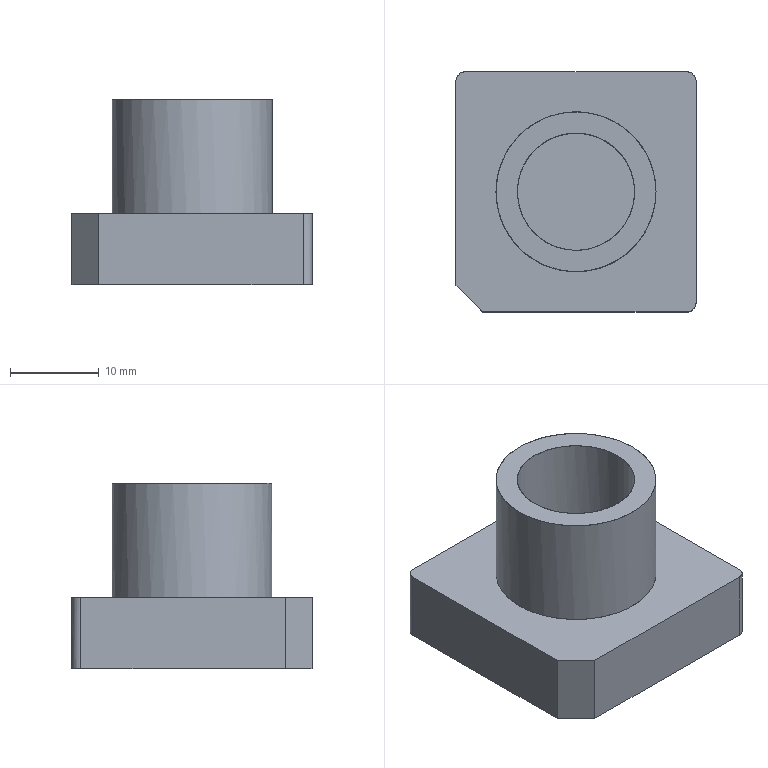NC program | PowerMill | posted with a generic post | part box 27 x 27 x 20.913 mm
Lines 15961 to 16766 of 92133:
N16058 M6
N16059 S8500 M03
N16060 G00 G90 X0.0 Y0.0
N16061 G43 Z11.803 H3
N16062
N16063 G05 P10000 R8
N16064 X19.2087 Y-4.6129
N16065 Z0.9326
N16066 G01 Z-0.2674 F360.0
N16067 X14.0835 Y-3.3645 F600.0
N16068 X1.7775 Y14.3702
N16069 X1.7498 Y14.3737
N16070 G03 X0.8293 Y14.4547 I-1.6397 J-13.3537
N16071 G01 X0.4792 Y14.472
N16072 G03 X-0.4792 I-0.4792 J-16.9289
N16073 G01 X-1.1152 Y14.4364
N16074 G03 X-2.0169 Y14.338 I1.0076 J-13.414
N16075 G01 X-2.3861 Y14.282
N16076 X-3.0221 Y14.1611
N16077 X-3.7382 Y13.9889
N16078 X-3.8175 Y13.9674
N16079 X11.7477 Y-8.4641
N16080 X11.5276 Y-8.7591
N16081 X11.3004 Y-9.0526
N16082 X11.0316 Y-9.379
N16083 X10.6658 Y-9.7933
N16084 X10.4003 Y-10.073
N16085 X10.1293 Y-10.3473
N16086 X9.7958 Y-10.6635
N16087 X9.4375 Y-10.9818
N16088 X9.0741 Y-11.284
N16089 X8.7582 Y-11.5288
N16090 X8.4375 Y-11.7672
N16091 X8.2539 Y-11.8951
N16092 X-8.2539 Y11.8951
N16093 X-8.4375 Y11.7672
N16094 X-8.7582 Y11.5288
N16095 X-9.0741 Y11.284
N16096 X-9.4375 Y10.9818
N16097 X-9.7958 Y10.6635
N16098 X-10.1293 Y10.3473
N16099 X-10.4003 Y10.073
N16100 X-10.6658 Y9.7933
N16101 X-11.0337 Y9.3766
N16102 X-11.2701 Y9.0893
N16103 X-11.6227 Y8.634
N16104 X-11.7476 Y8.464
N16105 X3.8175 Y-13.9674
N16106 X3.3294 Y-14.0906
N16107 X2.9954 Y-14.1667
N16108 X2.3861 Y-14.282
N16109 X2.0169 Y-14.338
N16110 G02 X1.1152 Y-14.4364 I-1.9093 J13.3156
N16111 G01 X0.4792 Y-14.472
N16112 G02 X-0.4792 I-0.4792 J16.9289
N16113 G01 X-0.8293 Y-14.4547
N16114 G02 X-1.7498 Y-14.3737 I0.7192 J13.4347
N16115 G01 X-1.7775 Y-14.3702
N16116 X-14.0835 Y3.3645
N16117 G00 Z11.803
N16118 G05 P0
N16119 (---------------)
N16120 ( END TOOLPATH : 精公基准台01-平坦面平行-D10 )
N16121 (---------------)
N16122 ( START TOOLPATH : 精公基准台01-基准面偏置-D10 )
N16123 (---------------)
N16124 G00 X0.0 Y0.0 Z9.8026
N16125 G05 P10000 R8
N16126 X8.5669 Y-24.255
N16127 Z-11.91
N16128 G01 Z-13.11 F360.0
N16129 Y-18.98 F600.0
N16130 X10.992 Y-9.2715
N16131 X10.7303 Y-9.5708
N16132 X10.4625 Y-9.8647
N16133 X10.1631 Y-10.1736
N16134 X9.8647 Y-10.4616
N16135 X9.5828 Y-10.7217
N16136 X9.301 Y-10.967
N16137 X9.0041 Y-11.2119
N16138 X8.5584 Y-11.5557
N16139 X8.1736 Y-11.8293
N16140 X7.6099 Y-12.2006
N16141 X7.0462 Y-12.5356
N16142 X6.766 Y-12.6888
N16143 X6.4825 Y-12.8359
N16144 X5.9188 Y-13.1045
N16145 X5.5954 Y-13.2468
N16146 X5.3551 Y-13.3443
N16147 X4.7914 Y-13.5567
N16148 X4.2277 Y-13.7442
N16149 X4.007 Y-13.8105
N16150 X3.664 Y-13.9055
N16151 X3.1003 Y-14.0414
N16152 X2.5366 Y-14.1546
N16153 X1.9729 Y-14.244
N16154 X1.4092 Y-14.3106
N16155 X0.8455 Y-14.3544
N16156 X0.2818 Y-14.3772
N16157 X-0.2818
N16158 X-0.8455 Y-14.3544
N16159 X-1.4092 Y-14.3106
N16160 X-1.9729 Y-14.244
N16161 X-2.5366 Y-14.1546
N16162 X-3.1003 Y-14.0414
N16163 X-3.664 Y-13.9055
N16164 X-4.007 Y-13.8105
N16165 X-4.2277 Y-13.7442
N16166 X-4.7914 Y-13.5567
N16167 X-5.3551 Y-13.3443
N16168 X-5.5954 Y-13.2468
N16169 X-5.9188 Y-13.1045
N16170 X-6.4825 Y-12.8359
N16171 X-6.766 Y-12.6888
N16172 X-7.0462 Y-12.5356
N16173 X-7.6099 Y-12.2006
N16174 X-8.1736 Y-11.8293
N16175 X-8.5584 Y-11.5557
N16176 X-9.0041 Y-11.2119
N16177 X-9.301 Y-10.967
N16178 X-9.5828 Y-10.7217
N16179 X-9.8647 Y-10.4616
N16180 X-10.1638 Y-10.1726
N16181 X-10.4625 Y-9.8647
N16182 X-10.7176 Y-9.5852
N16183 X-10.9673 Y-9.301
N16184 X-11.2114 Y-9.0034
N16185 X-11.4211 Y-8.7373
N16186 X-11.5557 Y-8.557
N16187 X-11.831 Y-8.1736
N16188 X-12.1194 Y-7.7392
N16189 X-12.2012 Y-7.6099
N16190 X-12.5356 Y-7.0462
N16191 X-12.8362 Y-6.4825
N16192 X-13.1056 Y-5.9188
N16193 X-13.2468 Y-5.5948
N16194 X-13.3454 Y-5.3551
N16195 X-13.557 Y-4.7914
N16196 X-13.7431 Y-4.2277
N16197 X-13.8105 Y-4.007
N16198 X-13.9044 Y-3.664
N16199 X-14.0414 Y-3.1003
N16200 X-14.1546 Y-2.5366
N16201 X-14.244 Y-1.9729
N16202 X-14.3106 Y-1.4092
N16203 X-14.3544 Y-0.8455
N16204 X-14.3761 Y-0.2818
N16205 X-14.3742 Y0.3875
N16206 X-14.3544 Y0.8455
N16207 X-14.3106 Y1.4092
N16208 X-14.244 Y1.9729
N16209 X-14.1546 Y2.5366
N16210 X-14.0414 Y3.1003
N16211 X-13.9044 Y3.664
N16212 X-13.8105 Y4.007
N16213 X-13.7431 Y4.2277
N16214 X-13.557 Y4.7914
N16215 X-13.3454 Y5.3551
N16216 X-13.2468 Y5.5948
N16217 X-13.1056 Y5.9188
N16218 X-12.8362 Y6.4825
N16219 X-12.5356 Y7.0462
N16220 X-12.2012 Y7.6099
N16221 X-12.1194 Y7.7392
N16222 X-11.831 Y8.1736
N16223 X-11.5557 Y8.557
N16224 X-11.4211 Y8.7373
N16225 X-11.2114 Y9.0034
N16226 X-10.9673 Y9.301
N16227 X-10.7176 Y9.5852
N16228 X-10.4625 Y9.8647
N16229 X-10.1736 Y10.1631
N16230 X-9.8647 Y10.4616
N16231 X-9.5828 Y10.7218
N16232 X-9.301 Y10.967
N16233 X-9.0041 Y11.2122
N16234 X-8.5584 Y11.5557
N16235 X-8.1736 Y11.8293
N16236 X-7.9552 Y11.9794
N16237 X-7.6099 Y12.2006
N16238 X-7.0462 Y12.5356
N16239 X-6.766 Y12.6888
N16240 X-6.4825 Y12.8359
N16241 X-5.9188 Y13.1045
N16242 X-5.5954 Y13.2468
N16243 X-5.0732 Y13.4556
N16244 X-4.7914 Y13.5567
N16245 X-4.2277 Y13.7442
N16246 X-4.007 Y13.8105
N16247 X-3.664 Y13.9055
N16248 X-3.1003 Y14.0414
N16249 X-2.5366 Y14.1546
N16250 X-1.9729 Y14.244
N16251 X-1.4092 Y14.3106
N16252 X-0.8455 Y14.3544
N16253 X-0.2818 Y14.3772
N16254 X0.2818
N16255 X0.8455 Y14.3544
N16256 X1.4092 Y14.3106
N16257 X1.9729 Y14.244
N16258 X2.5366 Y14.1546
N16259 X3.1003 Y14.0414
N16260 X3.664 Y13.9055
N16261 X4.007 Y13.8105
N16262 X4.2277 Y13.7442
N16263 X4.7914 Y13.5567
N16264 X5.0732 Y13.4556
N16265 X5.5954 Y13.2468
N16266 X5.9188 Y13.1045
N16267 X6.4825 Y12.8359
N16268 X6.766 Y12.6888
N16269 X7.0462 Y12.5356
N16270 X7.6099 Y12.2006
N16271 X7.9552 Y11.9794
N16272 X8.1736 Y11.8293
N16273 X8.5584 Y11.5557
N16274 X9.0034 Y11.2127
N16275 X9.301 Y10.967
N16276 X9.5828 Y10.7218
N16277 X9.8647 Y10.4616
N16278 X10.1734 Y10.1631
N16279 X10.4625 Y9.8647
N16280 X10.7174 Y9.5851
N16281 X10.9673 Y9.301
N16282 X11.2118 Y9.0034
N16283 X11.4211 Y8.7373
N16284 X11.5557 Y8.557
N16285 X11.831 Y8.1736
N16286 X12.1194 Y7.7392
N16287 X12.2012 Y7.6099
N16288 X12.5356 Y7.0462
N16289 X12.8362 Y6.4825
N16290 X13.1056 Y5.9188
N16291 X13.2468 Y5.5948
N16292 X13.3454 Y5.3551
N16293 X13.557 Y4.7914
N16294 X13.7431 Y4.2277
N16295 X13.8105 Y4.007
N16296 X13.9044 Y3.664
N16297 X14.0414 Y3.1003
N16298 X14.1546 Y2.5366
N16299 X14.244 Y1.9729
N16300 X14.3106 Y1.4092
N16301 X14.3544 Y0.8455
N16302 X14.3761 Y0.2818
N16303 X14.3742 Y-0.3875
N16304 X14.3544 Y-0.8455
N16305 X14.3106 Y-1.4092
N16306 X14.244 Y-1.9729
N16307 X14.1546 Y-2.5366
N16308 X14.0414 Y-3.1003
N16309 X13.9044 Y-3.664
N16310 X13.8105 Y-4.007
N16311 X13.7431 Y-4.2277
N16312 X13.557 Y-4.7914
N16313 X13.3454 Y-5.3551
N16314 X13.2468 Y-5.5948
N16315 X13.1056 Y-5.9188
N16316 X12.8362 Y-6.4825
N16317 X12.5356 Y-7.0462
N16318 X12.2012 Y-7.6099
N16319 X12.1194 Y-7.7392
N16320 X11.831 Y-8.1736
N16321 X11.5557 Y-8.557
N16322 X11.4211 Y-8.7373
N16323 X10.992 Y-9.2715
N16324 G00 Z9.8026
N16325 G05 P0
N16326 (---------------)
N16327 ( END TOOLPATH : 精公基准台01-基准面偏置-D10 )
N16328 (---------------)
N16329 ( START TOOLPATH : 精公基准台01-外形侧光-D10 )
N16330 (---------------)
N16331 G00 X0.0 Y0.0 Z10.803
N16332 G05 P10000 R8
N16333 X10.9671 Y-9.4667
N16334 Z-11.88
N16335 G01 Z-13.08 F360.0
N16336 G03 X9.9064 Y-9.906 I0.0 J-1.5 F600.0
N16337 G02 X-9.4563 Y-10.3368 I-9.9065 J9.9064
N16338 G02 X-10.4997 Y-9.2721 I8.9996 J9.8634
N16339 G02 X-12.4968 Y-6.3332 I10.3361 J9.1718
N16340 G02 X12.9211 Y5.4152 I12.4972 J6.3324
N16341 G02 X9.9064 Y-9.906 I-12.9212 J-5.4148
N16342 G03 X9.4671 Y-10.9667 I1.0606 J-1.0607
N16343 G01 X10.9106 Y-9.4101
N16344 G03 X9.85 Y-9.8494 I0.0001 J-1.5
N16345 G02 X-9.4016 Y-10.2784 I-9.8501 J9.8496
N16346 G02 X-10.4398 Y-9.2191 I8.9455 J9.8055
N16347 G02 X-12.4249 Y-6.2982 I10.2761 J9.1188
N16348 G02 X12.8702 Y5.329 I12.425 J6.2977
N16349 G02 X9.85 Y-9.8494 I-12.8703 J-5.3288
N16350 G03 X9.4107 Y-10.9101 I1.0607 J-1.0607
N16351 G00 Z10.803
N16352 G05 P0
N16353 (---------------)
N16354 ( END TOOLPATH : 精公基准台01-外形侧光-D10 )
N16355 (---------------)
N16356 ( START TOOLPATH : 精公基准台01-基准台侧光-D10 )
N16357 (---------------)
N16358 G00 X0.0 Y0.0 Z9.8026
N16359 G05 P10000 R8
N16360 X18.8035 Y-21.611
N16361 Z-19.81
N16362 G01 Z-21.01 F360.0
N16363 G03 X15.9877 Y-17.4792 I-1.4079 J2.0659 F600.0
N16364 G01 X15.8523 Y-17.5715
N16365 X15.8509 Y-17.5724
N16366 X15.8494 Y-17.5734
N16367 X15.5333 Y-17.7693
N16368 X15.5311 Y-17.7706
N16369 X15.5289 Y-17.7718
N16370 X15.2128 Y-17.9412
N16371 X15.2107 Y-17.9423
N16372 X15.2086 Y-17.9433
N16373 X14.8924 Y-18.0894
N16374 X14.8903 Y-18.0903
N16375 X14.8882 Y-18.0912
N16376 X14.5721 Y-18.216
N16377 X14.57 Y-18.2168
N16378 X14.5678 Y-18.2175
N16379 X14.2517 Y-18.3222
N16380 X14.2495 Y-18.3229
N16381 X14.2473 Y-18.3235
N16382 X13.9121 Y-18.4137
N16383 X13.9099 Y-18.4142
N16384 X13.9078 Y-18.4147
N16385 X13.6107 Y-18.4772
N16386 X13.6088 Y-18.4776
N16387 X13.6069 Y-18.478
N16388 X13.2907 Y-18.5283
N16389 X13.2885 Y-18.5287
N16390 X13.2863 Y-18.5289
N16391 X12.9701 Y-18.5614
N16392 X12.9681 Y-18.5615
N16393 X12.966 Y-18.5617
N16394 X12.6499 Y-18.5778
N16395 X12.6481
N16396 X12.6464 Y-18.5779
N16397 X12.3302 Y-18.58
N16398 X12.33
N16399 X12.3297
N16400 X-10.4328
N16401 X-10.4336
N16402 X-10.4344
N16403 X-10.7505 Y-18.5738
N16404 X-10.753 Y-18.5737
N16405 X-10.7555 Y-18.5735
N16406 X-11.0716 Y-18.5477
N16407 X-11.0742 Y-18.5475
N16408 X-11.0767 Y-18.5471
N16409 X-11.3928 Y-18.5009
N16410 X-11.3954 Y-18.5005
N16411 X-11.3979 Y-18.5
N16412 X-11.714 Y-18.4328
N16413 X-11.7166 Y-18.4322
N16414 X-11.7191 Y-18.4315
N16415 X-12.0352 Y-18.3424
N16416 X-12.0378 Y-18.3417
N16417 X-12.0403 Y-18.3408
N16418 X-12.3564 Y-18.2286
N16419 X-12.359 Y-18.2277
N16420 X-12.3614 Y-18.2266
N16421 X-12.6688 Y-18.0937
N16422 X-12.6713 Y-18.0926
N16423 X-12.6738 Y-18.0913
N16424 X-12.9988 Y-17.9229
N16425 X-13.0014 Y-17.9215
N16426 X-13.0039 Y-17.92
N16427 X-13.3201 Y-17.7253
N16428 X-13.3226 Y-17.7237
N16429 X-13.3251 Y-17.7219
N16430 X-13.6413 Y-17.4923
N16431 X-13.6439 Y-17.4903
N16432 X-13.6463 Y-17.4883
N16433 X-13.9625 Y-17.2171
N16434 X-13.9641 Y-17.2157
N16435 X-13.9657 Y-17.2142
N16436 X-14.0541 Y-17.1297
N16437 X-14.0548 Y-17.1291
N16438 X-14.0554 Y-17.1284
N16439 X-17.1284 Y-14.0554
N16440 X-17.1291 Y-14.0548
N16441 X-17.1297 Y-14.0541
N16442 X-17.2142 Y-13.9657
N16443 X-17.2155 Y-13.9643
N16444 X-17.2168 Y-13.9629
N16445 X-17.4484 Y-13.6963
N16446 X-17.4505 Y-13.6938
N16447 X-17.4524 Y-13.6912
N16448 X-17.7216 Y-13.3255
N16449 X-17.7235 Y-13.3228
N16450 X-17.7253 Y-13.3201
N16451 X-17.92 Y-13.0039
N16452 X-17.9215 Y-13.0014
N16453 X-17.9229 Y-12.9989
N16454 X-18.0871 Y-12.6827
N16455 X-18.0884 Y-12.6802
N16456 X-18.0895 Y-12.6776
N16457 X-18.2266 Y-12.3615
N16458 X-18.2276 Y-12.359
N16459 X-18.2286 Y-12.3564
N16460 X-18.3408 Y-12.0403
N16461 X-18.3416 Y-12.0381
N16462 X-18.3423 Y-12.0358
N16463 X-18.4133 Y-11.7906
N16464 X-18.414 Y-11.7881
N16465 X-18.4146 Y-11.7856
N16466 X-18.4999 Y-11.3985
N16467 X-18.5004 Y-11.3956
N16468 X-18.5009 Y-11.3928
N16469 X-18.5471 Y-11.0767
N16470 X-18.5475 Y-11.0742
N16471 X-18.5477 Y-11.0716
N16472 X-18.5735 Y-10.7555
N16473 X-18.5737 Y-10.753
N16474 X-18.5738 Y-10.7505
N16475 X-18.58 Y-10.4344
N16476 Y-10.4336
N16477 Y-10.4328
N16478 Y12.3297
N16479 Y12.33
N16480 Y12.3302
N16481 X-18.5779 Y12.6464
N16482 X-18.5778 Y12.6481
N16483 Y12.6498
N16484 X-18.5621 Y12.9659
N16485 X-18.562 Y12.9681
N16486 X-18.5618 Y12.9702
N16487 X-18.5289 Y13.2864
N16488 X-18.5287 Y13.2885
N16489 X-18.5284 Y13.2906
N16490 X-18.4783 Y13.6068
N16491 X-18.478 Y13.6088
N16492 X-18.4776 Y13.6108
N16493 X-18.4147 Y13.9079
N16494 X-18.4142 Y13.91
N16495 X-18.4137 Y13.9122
N16496 X-18.3235 Y14.2473
N16497 X-18.3228 Y14.2496
N16498 X-18.3221 Y14.2518
N16499 X-18.217 Y14.5679
N16500 X-18.2164 Y14.5699
N16501 X-18.2156 Y14.5719
N16502 X-18.0948 Y14.8799
N16503 X-18.0939 Y14.8821
N16504 X-18.0929 Y14.8843
N16505 X-17.9428 Y15.2086
N16506 X-17.9418 Y15.2106
N16507 X-17.9408 Y15.2127
N16508 X-17.7747 Y15.5238
N16509 X-17.7735 Y15.5259
N16510 X-17.7723 Y15.5281
N16511 X-17.5743 Y15.8493
N16512 X-17.5732 Y15.8509
N16513 X-17.5721 Y15.8525
N16514 X-17.454 Y16.0248
N16515 X-17.4532 Y16.0259
N16516 X-17.4525 Y16.0269
N16517 X-17.3468 Y16.1708
N16518 X-17.3458 Y16.1722
N16519 X-17.3447 Y16.1735
N16520 X-17.1342 Y16.4357
N16521 X-17.1325 Y16.4377
N16522 X-17.1308 Y16.4397
N16523 X-16.8146 Y16.7837
N16524 X-16.8125 Y16.7858
N16525 X-16.8104 Y16.788
N16526 X-16.4942 Y17.0837
N16527 X-16.4922 Y17.0855
N16528 X-16.49 Y17.0873
N16529 X-16.1739 Y17.3444
N16530 X-16.1724 Y17.3456
N16531 X-16.1708 Y17.3468
N16532 X-16.0268 Y17.4525
N16533 X-16.0257 Y17.4533
N16534 X-16.0245 Y17.4541
N16535 X-15.8523 Y17.5715
N16536 X-15.8509 Y17.5724
N16537 X-15.8494 Y17.5734
N16538 X-15.5333 Y17.7693
N16539 X-15.5311 Y17.7706
N16540 X-15.5289 Y17.7718
N16541 X-15.2128 Y17.9412
N16542 X-15.2107 Y17.9423
N16543 X-15.2086 Y17.9433
N16544 X-14.8924 Y18.0894
N16545 X-14.8903 Y18.0903
N16546 X-14.8882 Y18.0912
N16547 X-14.5721 Y18.216
N16548 X-14.57 Y18.2168
N16549 X-14.5678 Y18.2175
N16550 X-14.2517 Y18.3222
N16551 X-14.2496 Y18.3228
N16552 X-14.2475 Y18.3234
N16553 X-13.9313 Y18.4091
N16554 X-13.9292 Y18.4096
N16555 X-13.927 Y18.4101
N16556 X-13.6109 Y18.4772
N16557 X-13.6089 Y18.4776
N16558 X-13.6069 Y18.478
N16559 X-13.2907 Y18.5283
N16560 X-13.2885 Y18.5287
N16561 X-13.2863 Y18.5289
N16562 X-12.9701 Y18.5614
N16563 X-12.9681 Y18.5615
N16564 X-12.966 Y18.5617
N16565 X-12.6499 Y18.5778
N16566 X-12.6481
N16567 X-12.6464 Y18.5779
N16568 X-12.3302 Y18.58
N16569 X-12.33
N16570 X-12.3297
N16571 X0.0
N16572 X12.3297
N16573 X12.33
N16574 X12.3302
N16575 X12.6464 Y18.5779
N16576 X12.6481 Y18.5778
N16577 X12.6498
N16578 X12.9659 Y18.5621
N16579 X12.9681 Y18.562
N16580 X12.9702 Y18.5618
N16581 X13.2864 Y18.5289
N16582 X13.2885 Y18.5287
N16583 X13.2906 Y18.5284
N16584 X13.6068 Y18.4783
N16585 X13.6088 Y18.478
N16586 X13.6108 Y18.4776
N16587 X13.9079 Y18.4147
N16588 X13.91 Y18.4142
N16589 X13.9122 Y18.4137
N16590 X14.2473 Y18.3235
N16591 X14.2496 Y18.3228
N16592 X14.2518 Y18.3221
N16593 X14.5679 Y18.217
N16594 X14.5699 Y18.2164
N16595 X14.5719 Y18.2156
N16596 X14.8799 Y18.0948
N16597 X14.8821 Y18.0939
N16598 X14.8843 Y18.0929
N16599 X15.2086 Y17.9428
N16600 X15.2106 Y17.9418
N16601 X15.2127 Y17.9408
N16602 X15.5238 Y17.7747
N16603 X15.5259 Y17.7735
N16604 X15.5281 Y17.7723
N16605 X15.8493 Y17.5743
N16606 X15.8509 Y17.5732
N16607 X15.8525 Y17.5721
N16608 X16.0248 Y17.454
N16609 X16.0259 Y17.4532
N16610 X16.0269 Y17.4525
N16611 X16.1708 Y17.3468
N16612 X16.1722 Y17.3458
N16613 X16.1735 Y17.3447
N16614 X16.4357 Y17.1342
N16615 X16.4377 Y17.1325
N16616 X16.4397 Y17.1308
N16617 X16.7837 Y16.8146
N16618 X16.7858 Y16.8125
N16619 X16.788 Y16.8104
N16620 X17.0837 Y16.4942
N16621 X17.0855 Y16.4922
N16622 X17.0873 Y16.49
N16623 X17.3444 Y16.1739
N16624 X17.3456 Y16.1724
N16625 X17.3468 Y16.1708
N16626 X17.4525 Y16.0268
N16627 X17.4533 Y16.0257
N16628 X17.4541 Y16.0245
N16629 X17.5715 Y15.8523
N16630 X17.5724 Y15.8509
N16631 X17.5734 Y15.8494
N16632 X17.7693 Y15.5333
N16633 X17.7706 Y15.5311
N16634 X17.7718 Y15.5289
N16635 X17.9412 Y15.2128
N16636 X17.9423 Y15.2107
N16637 X17.9433 Y15.2086
N16638 X18.0894 Y14.8924
N16639 X18.0903 Y14.8903
N16640 X18.0912 Y14.8882
N16641 X18.216 Y14.5721
N16642 X18.2168 Y14.57
N16643 X18.2175 Y14.5678
N16644 X18.3222 Y14.2517
N16645 X18.3228 Y14.2496
N16646 X18.3234 Y14.2475
N16647 X18.4091 Y13.9313
N16648 X18.4096 Y13.9292
N16649 X18.4101 Y13.927
N16650 X18.4772 Y13.6109
N16651 X18.4776 Y13.6089
N16652 X18.478 Y13.6069
N16653 X18.5283 Y13.2907
N16654 X18.5287 Y13.2885
N16655 X18.5289 Y13.2863
N16656 X18.5614 Y12.9701
N16657 X18.5615 Y12.9681
N16658 X18.5617 Y12.966
N16659 X18.5778 Y12.6499
N16660 Y12.6481
N16661 X18.5779 Y12.6464
N16662 X18.58 Y12.3302
N16663 Y12.33
N16664 Y12.3297
N16665 Y-12.3297
N16666 Y-12.33
N16667 Y-12.3302
N16668 X18.5779 Y-12.6464
N16669 X18.5778 Y-12.6481
N16670 Y-12.6498
N16671 X18.5621 Y-12.9659
N16672 X18.562 Y-12.9681
N16673 X18.5618 Y-12.9702
N16674 X18.5289 Y-13.2864
N16675 X18.5287 Y-13.2885
N16676 X18.5284 Y-13.2906
N16677 X18.4783 Y-13.6068
N16678 X18.478 Y-13.6088
N16679 X18.4776 Y-13.6108
N16680 X18.4147 Y-13.9079
N16681 X18.4142 Y-13.91
N16682 X18.4137 Y-13.9122
N16683 X18.3235 Y-14.2473
N16684 X18.3228 Y-14.2496
N16685 X18.3221 Y-14.2518
N16686 X18.217 Y-14.5679
N16687 X18.2164 Y-14.5699
N16688 X18.2156 Y-14.5719
N16689 X18.0948 Y-14.8799
N16690 X18.0939 Y-14.8821
N16691 X18.0929 Y-14.8843
N16692 X17.9428 Y-15.2086
N16693 X17.9418 Y-15.2106
N16694 X17.9408 Y-15.2127
N16695 X17.7747 Y-15.5238
N16696 X17.7735 Y-15.5259
N16697 X17.7723 Y-15.5281
N16698 X17.5743 Y-15.8493
N16699 X17.5732 Y-15.8509
N16700 X17.5721 Y-15.8525
N16701 X17.454 Y-16.0248
N16702 X17.4532 Y-16.0259
N16703 X17.4525 Y-16.0269
N16704 X17.3468 Y-16.1708
N16705 X17.3458 Y-16.1722
N16706 X17.3447 Y-16.1735
N16707 X17.1342 Y-16.4357
N16708 X17.1325 Y-16.4377
N16709 X17.1308 Y-16.4397
N16710 X16.8146 Y-16.7837
N16711 X16.8125 Y-16.7858
N16712 X16.8104 Y-16.788
N16713 X16.4942 Y-17.0837
N16714 X16.4922 Y-17.0855
N16715 X16.49 Y-17.0873
N16716 X16.1739 Y-17.3444
N16717 X16.1724 Y-17.3456
N16718 X16.1708 Y-17.3468
N16719 X16.0268 Y-17.4525
N16720 X16.0257 Y-17.4533
N16721 X16.0245 Y-17.4541
N16722 X15.9877 Y-17.4792
N16723 G03 X18.8034 Y-21.611 I1.4079 J-2.0659
N16724 G01 X18.752 Y-21.5493
N16725 G03 X15.9362 Y-17.4175 I-1.4079 J2.0659
N16726 G01 X15.8073 Y-17.5054
N16727 X15.4911 Y-17.7013
N16728 X15.175 Y-17.8707
N16729 X14.8588 Y-18.0168
N16730 X14.5427 Y-18.1416
N16731 X14.2266 Y-18.2462
N16732 X13.8913 Y-18.3364
N16733 X13.5943 Y-18.399
N16734 X13.2781 Y-18.4493
N16735 X12.962 Y-18.4818
N16736 X12.6458 Y-18.4979
N16737 X12.3297 Y-18.5
N16738 X-10.4328
N16739 X-10.749 Y-18.4938
N16740 X-11.0651 Y-18.468
N16741 X-11.3812 Y-18.4217
N16742 X-11.6974 Y-18.3545
N16743 X-12.0135 Y-18.2654
N16744 X-12.3297 Y-18.1532
N16745 X-12.637 Y-18.0203
N16746 X-12.962 Y-17.8519
N16747 X-13.2781 Y-17.6572
N16748 X-13.5943 Y-17.4275
N16749 X-13.9104 Y-17.1564
N16750 X-13.9988 Y-17.0719
N16751 X-17.0719 Y-13.9988
N16752 X-17.1564 Y-13.9104
N16753 X-17.388 Y-13.6438
N16754 X-17.6572 Y-13.2781
N16755 X-17.8519 Y-12.962
N16756 X-18.0161 Y-12.6458
N16757 X-18.1532 Y-12.3297
N16758 X-18.2654 Y-12.0135
N16759 X-18.3364 Y-11.7684
N16760 X-18.4217 Y-11.3812
N16761 X-18.468 Y-11.0651
N16762 X-18.4938 Y-10.749
N16763 X-18.5 Y-10.4328
N16764 Y12.3297
N16765 X-18.4979 Y12.6458
N16766 X-18.4822 Y12.962
N16767 X-18.4493 Y13.2781
N16768 X-18.3993 Y13.5943
N16769 X-18.3364 Y13.8914
N16770 X-18.2462 Y14.2266
N16771 X-18.1411 Y14.5427
N16772 X-18.0203 Y14.8507
N16773 X-17.8702 Y15.175
N16774 X-17.7042 Y15.4861
N16775 X-17.5062 Y15.8073
N16776 X-17.388 Y15.9796
N16777 X-17.2823 Y16.1234
N16778 X-17.0719 Y16.3856
N16779 X-16.7557 Y16.7295
N16780 X-16.4396 Y17.0252
N16781 X-16.1234 Y17.2823
N16782 X-15.9795 Y17.388
N16783 X-15.8073 Y17.5054
N16784 X-15.4911 Y17.7013
N16785 X-15.175 Y17.8707
N16786 X-14.8588 Y18.0168
N16787 X-14.5427 Y18.1416
N16788 X-14.2266 Y18.2462
N16789 X-13.9104 Y18.3318
N16790 X-13.5943 Y18.399
N16791 X-13.2781 Y18.4493
N16792 X-12.962 Y18.4818
N16793 X-12.6458 Y18.4979
N16794 X-12.3297 Y18.5
N16795 X0.0
N16796 X12.3297
N16797 X12.6458 Y18.4979
N16798 X12.962 Y18.4822
N16799 X13.2781 Y18.4493
N16800 X13.5943 Y18.3993
N16801 X13.8914 Y18.3364
N16802 X14.2266 Y18.2462
N16803 X14.5427 Y18.1411
N16804 X14.8507 Y18.0203
N16805 X15.175 Y17.8702
N16806 X15.4861 Y17.7042
N16807 X15.8073 Y17.5062
N16808 X15.9796 Y17.388
N16809 X16.1234 Y17.2823
N16810 X16.3856 Y17.0719
N16811 X16.7295 Y16.7557
N16812 X17.0252 Y16.4396
N16813 X17.2823 Y16.1234
N16814 X17.388 Y15.9795
N16815 X17.5054 Y15.8073
N16816 X17.7013 Y15.4911
N16817 X17.8707 Y15.175
N16818 X18.0168 Y14.8588
N16819 X18.1416 Y14.5427
N16820 X18.2462 Y14.2266
N16821 X18.3318 Y13.9104
N16822 X18.399 Y13.5943
N16823 X18.4493 Y13.2781
N16824 X18.4818 Y12.962
N16825 X18.4979 Y12.6458
N16826 X18.5 Y12.3297
N16827 Y-12.3297
N16828 X18.4979 Y-12.6458
N16829 X18.4822 Y-12.962
N16830 X18.4493 Y-13.2781
N16831 X18.3993 Y-13.5943
N16832 X18.3364 Y-13.8914
N16833 X18.2462 Y-14.2266
N16834 X18.1411 Y-14.5427
N16835 X18.0203 Y-14.8507
N16836 X17.8702 Y-15.175
N16837 X17.7042 Y-15.4861
N16838 X17.5062 Y-15.8073
N16839 X17.388 Y-15.9796
N16840 X17.2823 Y-16.1234
N16841 X17.0719 Y-16.3856
N16842 X16.7557 Y-16.7295
N16843 X16.4396 Y-17.0252
N16844 X16.1234 Y-17.2823
N16845 X15.9795 Y-17.388
N16846 X15.9362 Y-17.4175
N16847 G03 X18.752 Y-21.5492 I1.4079 J-2.0659
N16848 G00 Z9.8026
N16849 G05 P0
N16850 (---------------)
N16851 ( END TOOLPATH : 精公基准台01-基准台侧光-D10 )
N16852 (---------------)
N16853
N16854 M05
N16855 G53 Z0.0
N16856 (---------------)
N16857 ( START TOOLPATH : 精公精光01-等高-D4 )
N16858 (---------------)
N16859 ( TOOL NO.    :14 )
N16860 ( TOOL TYPE   : ENDMILL)
N16861 ( TOOL ID     : D4_1_1)
N16862 ( TOOL DIA    : 4.0 LENGTH 66.84)
N16863 T14